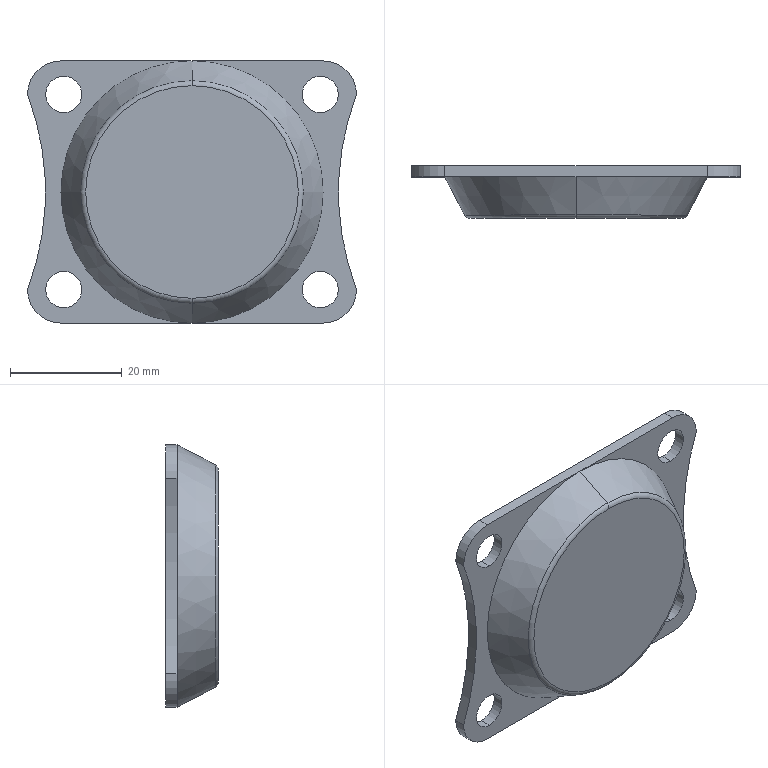Part | STEP file | CLGJ50_Rswivel | 1 solid | 27 faces | box 59 x 9.375 x 47 mm | volume 14515 mm3 | cylinder 16 | plane 7 | torus 2 | cone 2 | commonest cylinder face diameters 6.5 x8 12 x4 39.333 x2 98.33 x2
STEP:
#1=CARTESIAN_POINT('',(0.,-9.375,19.059));
#2=VERTEX_POINT('',#1);
#3=CARTESIAN_POINT('',(0.,-9.375,-19.059));
#4=VERTEX_POINT('',#3);
#5=CARTESIAN_POINT('',(0.,-9.375,0.));
#6=DIRECTION('',(0.,1.,0.));
#7=DIRECTION('',(0.,0.,1.));
#8=AXIS2_PLACEMENT_3D('',#5,#6,#7);
#9=CIRCLE('',#8,19.059);
#10=EDGE_CURVE('',#2,#4,#9,.T.);
#11=ORIENTED_EDGE('',*,*,#10,.T.);
#12=CARTESIAN_POINT('',(0.,-8.836,-19.947));
#13=VERTEX_POINT('',#12);
#14=CARTESIAN_POINT('',(0.,-8.375,-19.059));
#15=DIRECTION('',(1.,0.,0.));
#16=DIRECTION('',(0.,0.,-1.));
#17=AXIS2_PLACEMENT_3D('',#14,#15,#16);
#18=CIRCLE('',#17,1.);
#19=EDGE_CURVE('',#4,#13,#18,.T.);
#20=ORIENTED_EDGE('',*,*,#19,.T.);
#21=CARTESIAN_POINT('',(0.,-8.836,19.947));
#22=VERTEX_POINT('',#21);
#23=CARTESIAN_POINT('',(0.,-8.836,0.));
#24=DIRECTION('',(0.,1.,0.));
#25=DIRECTION('',(0.,0.,1.));
#26=AXIS2_PLACEMENT_3D('',#23,#24,#25);
#27=CIRCLE('',#26,19.947);
#28=EDGE_CURVE('',#22,#13,#27,.T.);
#29=ORIENTED_EDGE('',*,*,#28,.F.);
#30=CARTESIAN_POINT('',(0.,-8.375,19.059));
#31=DIRECTION('',(-1.,0.,0.));
#32=DIRECTION('',(0.,0.,1.));
#33=AXIS2_PLACEMENT_3D('',#30,#31,#32);
#34=CIRCLE('',#33,1.);
#35=EDGE_CURVE('',#2,#22,#34,.T.);
#36=ORIENTED_EDGE('',*,*,#35,.F.);
#37=EDGE_LOOP('',(#11,#20,#29,#36));
#38=FACE_OUTER_BOUND('',#37,.T.);
#39=CARTESIAN_POINT('',(0.,-8.375,0.));
#40=DIRECTION('',(0.,1.,0.));
#41=DIRECTION('',(0.,0.,1.));
#42=AXIS2_PLACEMENT_3D('',#39,#40,#41);
#43=TOROIDAL_SURFACE('',#42,19.059,1.);
#44=ADVANCED_FACE('',(#38),#43,.T.);
#45=ORIENTED_EDGE('',*,*,#28,.T.);
#46=CARTESIAN_POINT('',(0.,-2.,-23.5));
#47=VERTEX_POINT('',#46);
#48=CARTESIAN_POINT('',(0.,-8.836,-19.947));
#49=DIRECTION('',(0.,0.8873,-0.4612));
#50=VECTOR('',#49,1000.);
#51=LINE('',#48,#50);
#52=EDGE_CURVE('',#13,#47,#51,.T.);
#53=ORIENTED_EDGE('',*,*,#52,.T.);
#54=CARTESIAN_POINT('',(0.,-2.,23.5));
#55=VERTEX_POINT('',#54);
#56=CARTESIAN_POINT('',(0.,-2.,0.));
#57=DIRECTION('',(0.,1.,0.));
#58=DIRECTION('',(0.,0.,1.));
#59=AXIS2_PLACEMENT_3D('',#56,#57,#58);
#60=CIRCLE('',#59,23.5);
#61=EDGE_CURVE('',#55,#47,#60,.T.);
#62=ORIENTED_EDGE('',*,*,#61,.F.);
#63=CARTESIAN_POINT('',(0.,-8.836,19.947));
#64=DIRECTION('',(0.,0.8873,0.4612));
#65=VECTOR('',#64,1000.);
#66=LINE('',#63,#65);
#67=EDGE_CURVE('',#22,#55,#66,.T.);
#68=ORIENTED_EDGE('',*,*,#67,.F.);
#69=EDGE_LOOP('',(#45,#53,#62,#68));
#70=FACE_OUTER_BOUND('',#69,.T.);
#71=CARTESIAN_POINT('',(0.,-8.836,0.));
#72=DIRECTION('',(0.,1.,0.));
#73=DIRECTION('',(0.,0.,1.));
#74=AXIS2_PLACEMENT_3D('',#71,#72,#73);
#75=CONICAL_SURFACE('',#74,19.947,0.4793);
#76=ADVANCED_FACE('',(#70),#75,.T.);
#77=CARTESIAN_POINT('',(0.,-1.,-19.667));
#78=VERTEX_POINT('',#77);
#79=CARTESIAN_POINT('',(0.,-1.,19.667));
#80=VERTEX_POINT('',#79);
#81=CARTESIAN_POINT('',(0.,-1.,0.));
#82=DIRECTION('',(0.,1.,0.));
#83=DIRECTION('',(0.,0.,1.));
#84=AXIS2_PLACEMENT_3D('',#81,#82,#83);
#85=CIRCLE('',#84,19.667);
#86=EDGE_CURVE('',#78,#80,#85,.T.);
#87=ORIENTED_EDGE('',*,*,#86,.F.);
#88=CARTESIAN_POINT('',(0.,0.,-19.667));
#89=VERTEX_POINT('',#88);
#90=CARTESIAN_POINT('',(0.,-1.,-19.667));
#91=DIRECTION('',(0.,1.,0.));
#92=VECTOR('',#91,1000.);
#93=LINE('',#90,#92);
#94=EDGE_CURVE('',#78,#89,#93,.T.);
#95=ORIENTED_EDGE('',*,*,#94,.T.);
#96=CARTESIAN_POINT('',(0.,0.,19.667));
#97=VERTEX_POINT('',#96);
#98=CARTESIAN_POINT('',(0.,0.,0.));
#99=DIRECTION('',(0.,1.,0.));
#100=DIRECTION('',(0.,0.,1.));
#101=AXIS2_PLACEMENT_3D('',#98,#99,#100);
#102=CIRCLE('',#101,19.667);
#103=EDGE_CURVE('',#89,#97,#102,.T.);
#104=ORIENTED_EDGE('',*,*,#103,.T.);
#105=CARTESIAN_POINT('',(0.,-1.,19.667));
#106=DIRECTION('',(0.,1.,0.));
#107=VECTOR('',#106,1000.);
#108=LINE('',#105,#107);
#109=EDGE_CURVE('',#80,#97,#108,.T.);
#110=ORIENTED_EDGE('',*,*,#109,.F.);
#111=EDGE_LOOP('',(#87,#95,#104,#110));
#112=FACE_OUTER_BOUND('',#111,.T.);
#113=CARTESIAN_POINT('',(0.,-1.,0.));
#114=DIRECTION('',(0.,1.,0.));
#115=DIRECTION('',(0.,0.,1.));
#116=AXIS2_PLACEMENT_3D('',#113,#114,#115);
#117=CYLINDRICAL_SURFACE('',#116,19.667);
#118=ADVANCED_FACE('',(#112),#117,.F.);
#119=CARTESIAN_POINT('',(-23.,-2.,-20.75));
#120=VERTEX_POINT('',#119);
#121=CARTESIAN_POINT('',(-23.,-2.,-14.25));
#122=VERTEX_POINT('',#121);
#123=CARTESIAN_POINT('',(-23.,-2.,-17.5));
#124=DIRECTION('',(0.,1.,0.));
#125=DIRECTION('',(0.,0.,1.));
#126=AXIS2_PLACEMENT_3D('',#123,#124,#125);
#127=CIRCLE('',#126,3.25);
#128=EDGE_CURVE('',#120,#122,#127,.T.);
#129=ORIENTED_EDGE('',*,*,#128,.F.);
#130=CARTESIAN_POINT('',(-23.,0.,-20.75));
#131=VERTEX_POINT('',#130);
#132=CARTESIAN_POINT('',(-23.,-2.,-20.75));
#133=DIRECTION('',(0.,1.,0.));
#134=VECTOR('',#133,1000.);
#135=LINE('',#132,#134);
#136=EDGE_CURVE('',#120,#131,#135,.T.);
#137=ORIENTED_EDGE('',*,*,#136,.T.);
#138=CARTESIAN_POINT('',(-23.,0.,-14.25));
#139=VERTEX_POINT('',#138);
#140=CARTESIAN_POINT('',(-23.,0.,-17.5));
#141=DIRECTION('',(0.,1.,0.));
#142=DIRECTION('',(0.,0.,1.));
#143=AXIS2_PLACEMENT_3D('',#140,#141,#142);
#144=CIRCLE('',#143,3.25);
#145=EDGE_CURVE('',#131,#139,#144,.T.);
#146=ORIENTED_EDGE('',*,*,#145,.T.);
#147=CARTESIAN_POINT('',(-23.,-2.,-14.25));
#148=DIRECTION('',(0.,1.,0.));
#149=VECTOR('',#148,1000.);
#150=LINE('',#147,#149);
#151=EDGE_CURVE('',#122,#139,#150,.T.);
#152=ORIENTED_EDGE('',*,*,#151,.F.);
#153=EDGE_LOOP('',(#129,#137,#146,#152));
#154=FACE_OUTER_BOUND('',#153,.T.);
#155=CARTESIAN_POINT('',(-23.,-2.,-17.5));
#156=DIRECTION('',(0.,1.,0.));
#157=DIRECTION('',(0.,0.,1.));
#158=AXIS2_PLACEMENT_3D('',#155,#156,#157);
#159=CYLINDRICAL_SURFACE('',#158,3.25);
#160=ADVANCED_FACE('',(#154),#159,.F.);
#161=CARTESIAN_POINT('',(-23.,-2.,14.25));
#162=VERTEX_POINT('',#161);
#163=CARTESIAN_POINT('',(-23.,-2.,20.75));
#164=VERTEX_POINT('',#163);
#165=CARTESIAN_POINT('',(-23.,-2.,17.5));
#166=DIRECTION('',(0.,1.,0.));
#167=DIRECTION('',(0.,0.,1.));
#168=AXIS2_PLACEMENT_3D('',#165,#166,#167);
#169=CIRCLE('',#168,3.25);
#170=EDGE_CURVE('',#162,#164,#169,.T.);
#171=ORIENTED_EDGE('',*,*,#170,.F.);
#172=CARTESIAN_POINT('',(-23.,0.,14.25));
#173=VERTEX_POINT('',#172);
#174=CARTESIAN_POINT('',(-23.,-2.,14.25));
#175=DIRECTION('',(0.,1.,0.));
#176=VECTOR('',#175,1000.);
#177=LINE('',#174,#176);
#178=EDGE_CURVE('',#162,#173,#177,.T.);
#179=ORIENTED_EDGE('',*,*,#178,.T.);
#180=CARTESIAN_POINT('',(-23.,0.,20.75));
#181=VERTEX_POINT('',#180);
#182=CARTESIAN_POINT('',(-23.,0.,17.5));
#183=DIRECTION('',(0.,1.,0.));
#184=DIRECTION('',(0.,0.,1.));
#185=AXIS2_PLACEMENT_3D('',#182,#183,#184);
#186=CIRCLE('',#185,3.25);
#187=EDGE_CURVE('',#173,#181,#186,.T.);
#188=ORIENTED_EDGE('',*,*,#187,.T.);
#189=CARTESIAN_POINT('',(-23.,-2.,20.75));
#190=DIRECTION('',(0.,1.,0.));
#191=VECTOR('',#190,1000.);
#192=LINE('',#189,#191);
#193=EDGE_CURVE('',#164,#181,#192,.T.);
#194=ORIENTED_EDGE('',*,*,#193,.F.);
#195=EDGE_LOOP('',(#171,#179,#188,#194));
#196=FACE_OUTER_BOUND('',#195,.T.);
#197=CARTESIAN_POINT('',(-23.,-2.,17.5));
#198=DIRECTION('',(0.,1.,0.));
#199=DIRECTION('',(0.,0.,1.));
#200=AXIS2_PLACEMENT_3D('',#197,#198,#199);
#201=CYLINDRICAL_SURFACE('',#200,3.25);
#202=ADVANCED_FACE('',(#196),#201,.F.);
#203=CARTESIAN_POINT('',(23.,-2.,-20.75));
#204=VERTEX_POINT('',#203);
#205=CARTESIAN_POINT('',(23.,-2.,-14.25));
#206=VERTEX_POINT('',#205);
#207=CARTESIAN_POINT('',(23.,-2.,-17.5));
#208=DIRECTION('',(0.,1.,0.));
#209=DIRECTION('',(0.,0.,1.));
#210=AXIS2_PLACEMENT_3D('',#207,#208,#209);
#211=CIRCLE('',#210,3.25);
#212=EDGE_CURVE('',#204,#206,#211,.T.);
#213=ORIENTED_EDGE('',*,*,#212,.F.);
#214=CARTESIAN_POINT('',(23.,0.,-20.75));
#215=VERTEX_POINT('',#214);
#216=CARTESIAN_POINT('',(23.,-2.,-20.75));
#217=DIRECTION('',(0.,1.,0.));
#218=VECTOR('',#217,1000.);
#219=LINE('',#216,#218);
#220=EDGE_CURVE('',#204,#215,#219,.T.);
#221=ORIENTED_EDGE('',*,*,#220,.T.);
#222=CARTESIAN_POINT('',(23.,0.,-14.25));
#223=VERTEX_POINT('',#222);
#224=CARTESIAN_POINT('',(23.,0.,-17.5));
#225=DIRECTION('',(0.,1.,0.));
#226=DIRECTION('',(0.,0.,1.));
#227=AXIS2_PLACEMENT_3D('',#224,#225,#226);
#228=CIRCLE('',#227,3.25);
#229=EDGE_CURVE('',#215,#223,#228,.T.);
#230=ORIENTED_EDGE('',*,*,#229,.T.);
#231=CARTESIAN_POINT('',(23.,-2.,-14.25));
#232=DIRECTION('',(0.,1.,0.));
#233=VECTOR('',#232,1000.);
#234=LINE('',#231,#233);
#235=EDGE_CURVE('',#206,#223,#234,.T.);
#236=ORIENTED_EDGE('',*,*,#235,.F.);
#237=EDGE_LOOP('',(#213,#221,#230,#236));
#238=FACE_OUTER_BOUND('',#237,.T.);
#239=CARTESIAN_POINT('',(23.,-2.,-17.5));
#240=DIRECTION('',(0.,1.,0.));
#241=DIRECTION('',(0.,0.,1.));
#242=AXIS2_PLACEMENT_3D('',#239,#240,#241);
#243=CYLINDRICAL_SURFACE('',#242,3.25);
#244=ADVANCED_FACE('',(#238),#243,.F.);
#245=CARTESIAN_POINT('',(23.,-2.,14.25));
#246=VERTEX_POINT('',#245);
#247=CARTESIAN_POINT('',(23.,-2.,20.75));
#248=VERTEX_POINT('',#247);
#249=CARTESIAN_POINT('',(23.,-2.,17.5));
#250=DIRECTION('',(0.,1.,0.));
#251=DIRECTION('',(0.,0.,1.));
#252=AXIS2_PLACEMENT_3D('',#249,#250,#251);
#253=CIRCLE('',#252,3.25);
#254=EDGE_CURVE('',#246,#248,#253,.T.);
#255=ORIENTED_EDGE('',*,*,#254,.F.);
#256=CARTESIAN_POINT('',(23.,0.,14.25));
#257=VERTEX_POINT('',#256);
#258=CARTESIAN_POINT('',(23.,-2.,14.25));
#259=DIRECTION('',(0.,1.,0.));
#260=VECTOR('',#259,1000.);
#261=LINE('',#258,#260);
#262=EDGE_CURVE('',#246,#257,#261,.T.);
#263=ORIENTED_EDGE('',*,*,#262,.T.);
#264=CARTESIAN_POINT('',(23.,0.,20.75));
#265=VERTEX_POINT('',#264);
#266=CARTESIAN_POINT('',(23.,0.,17.5));
#267=DIRECTION('',(0.,1.,0.));
#268=DIRECTION('',(0.,0.,1.));
#269=AXIS2_PLACEMENT_3D('',#266,#267,#268);
#270=CIRCLE('',#269,3.25);
#271=EDGE_CURVE('',#257,#265,#270,.T.);
#272=ORIENTED_EDGE('',*,*,#271,.T.);
#273=CARTESIAN_POINT('',(23.,-2.,20.75));
#274=DIRECTION('',(0.,1.,0.));
#275=VECTOR('',#274,1000.);
#276=LINE('',#273,#275);
#277=EDGE_CURVE('',#248,#265,#276,.T.);
#278=ORIENTED_EDGE('',*,*,#277,.F.);
#279=EDGE_LOOP('',(#255,#263,#272,#278));
#280=FACE_OUTER_BOUND('',#279,.T.);
#281=CARTESIAN_POINT('',(23.,-2.,17.5));
#282=DIRECTION('',(0.,1.,0.));
#283=DIRECTION('',(0.,0.,1.));
#284=AXIS2_PLACEMENT_3D('',#281,#282,#283);
#285=CYLINDRICAL_SURFACE('',#284,3.25);
#286=ADVANCED_FACE('',(#280),#285,.F.);
#287=CARTESIAN_POINT('',(23.,-2.,17.5));
#288=DIRECTION('',(0.,1.,0.));
#289=DIRECTION('',(0.,0.,1.));
#290=AXIS2_PLACEMENT_3D('',#287,#288,#289);
#291=CIRCLE('',#290,3.25);
#292=EDGE_CURVE('',#248,#246,#291,.T.);
#293=ORIENTED_EDGE('',*,*,#292,.T.);
#294=ORIENTED_EDGE('',*,*,#254,.T.);
#295=EDGE_LOOP('',(#293,#294));
#296=FACE_BOUND('',#295,.T.);
#297=CARTESIAN_POINT('',(23.,-2.,-17.5));
#298=DIRECTION('',(0.,1.,0.));
#299=DIRECTION('',(0.,0.,1.));
#300=AXIS2_PLACEMENT_3D('',#297,#298,#299);
#301=CIRCLE('',#300,3.25);
#302=EDGE_CURVE('',#206,#204,#301,.T.);
#303=ORIENTED_EDGE('',*,*,#302,.T.);
#304=ORIENTED_EDGE('',*,*,#212,.T.);
#305=EDGE_LOOP('',(#303,#304));
#306=FACE_BOUND('',#305,.T.);
#307=CARTESIAN_POINT('',(23.5,-2.,23.5));
#308=VERTEX_POINT('',#307);
#309=CARTESIAN_POINT('',(-23.5,-2.,23.5));
#310=DIRECTION('',(1.,0.,0.));
#311=VECTOR('',#310,1000.);
#312=LINE('',#309,#311);
#313=EDGE_CURVE('',#55,#308,#312,.T.);
#314=ORIENTED_EDGE('',*,*,#313,.F.);
#315=ORIENTED_EDGE('',*,*,#61,.T.);
#316=CARTESIAN_POINT('',(23.5,-2.,-23.5));
#317=VERTEX_POINT('',#316);
#318=CARTESIAN_POINT('',(23.5,-2.,-23.5));
#319=DIRECTION('',(-1.,0.,0.));
#320=VECTOR('',#319,1000.);
#321=LINE('',#318,#320);
#322=EDGE_CURVE('',#317,#47,#321,.T.);
#323=ORIENTED_EDGE('',*,*,#322,.F.);
#324=CARTESIAN_POINT('',(29.5,-2.,-17.5));
#325=VERTEX_POINT('',#324);
#326=CARTESIAN_POINT('',(23.5,-2.,-17.5));
#327=DIRECTION('',(0.,1.,0.));
#328=DIRECTION('',(0.,0.,1.));
#329=AXIS2_PLACEMENT_3D('',#326,#327,#328);
#330=CIRCLE('',#329,6.);
#331=EDGE_CURVE('',#325,#317,#330,.T.);
#332=ORIENTED_EDGE('',*,*,#331,.F.);
#333=CARTESIAN_POINT('',(29.5,-2.,17.5));
#334=VERTEX_POINT('',#333);
#335=CARTESIAN_POINT('',(75.445,-2.,0.));
#336=DIRECTION('',(0.,-1.,0.));
#337=DIRECTION('',(0.,0.,-1.));
#338=AXIS2_PLACEMENT_3D('',#335,#336,#337);
#339=CIRCLE('',#338,49.165);
#340=EDGE_CURVE('',#334,#325,#339,.T.);
#341=ORIENTED_EDGE('',*,*,#340,.F.);
#342=CARTESIAN_POINT('',(23.5,-2.,17.5));
#343=DIRECTION('',(0.,1.,0.));
#344=DIRECTION('',(0.,0.,1.));
#345=AXIS2_PLACEMENT_3D('',#342,#343,#344);
#346=CIRCLE('',#345,6.);
#347=EDGE_CURVE('',#308,#334,#346,.T.);
#348=ORIENTED_EDGE('',*,*,#347,.F.);
#349=EDGE_LOOP('',(#314,#315,#323,#332,#341,#348));
#350=FACE_OUTER_BOUND('',#349,.T.);
#351=CARTESIAN_POINT('',(-23.5,-2.,-17.5));
#352=DIRECTION('',(0.,1.,0.));
#353=DIRECTION('',(0.,0.,1.));
#354=AXIS2_PLACEMENT_3D('',#351,#352,#353);
#355=PLANE('',#354);
#356=ADVANCED_FACE('',(#296,#306,#350),#355,.F.);
#357=CARTESIAN_POINT('',(-23.5,0.,-23.5));
#358=VERTEX_POINT('',#357);
#359=CARTESIAN_POINT('',(-29.5,0.,-17.5));
#360=VERTEX_POINT('',#359);
#361=CARTESIAN_POINT('',(-23.5,0.,-17.5));
#362=DIRECTION('',(0.,1.,0.));
#363=DIRECTION('',(0.,0.,1.));
#364=AXIS2_PLACEMENT_3D('',#361,#362,#363);
#365=CIRCLE('',#364,6.);
#366=EDGE_CURVE('',#358,#360,#365,.T.);
#367=ORIENTED_EDGE('',*,*,#366,.F.);
#368=CARTESIAN_POINT('',(-23.5,-2.,-23.5));
#369=VERTEX_POINT('',#368);
#370=CARTESIAN_POINT('',(-23.5,-2.,-23.5));
#371=DIRECTION('',(0.,1.,0.));
#372=VECTOR('',#371,1000.);
#373=LINE('',#370,#372);
#374=EDGE_CURVE('',#369,#358,#373,.T.);
#375=ORIENTED_EDGE('',*,*,#374,.F.);
#376=CARTESIAN_POINT('',(-29.5,-2.,-17.5));
#377=VERTEX_POINT('',#376);
#378=CARTESIAN_POINT('',(-23.5,-2.,-17.5));
#379=DIRECTION('',(0.,1.,0.));
#380=DIRECTION('',(0.,0.,1.));
#381=AXIS2_PLACEMENT_3D('',#378,#379,#380);
#382=CIRCLE('',#381,6.);
#383=EDGE_CURVE('',#369,#377,#382,.T.);
#384=ORIENTED_EDGE('',*,*,#383,.T.);
#385=CARTESIAN_POINT('',(-29.5,-2.,-17.5));
#386=DIRECTION('',(0.,1.,0.));
#387=VECTOR('',#386,1000.);
#388=LINE('',#385,#387);
#389=EDGE_CURVE('',#377,#360,#388,.T.);
#390=ORIENTED_EDGE('',*,*,#389,.T.);
#391=EDGE_LOOP('',(#367,#375,#384,#390));
#392=FACE_OUTER_BOUND('',#391,.T.);
#393=CARTESIAN_POINT('',(-23.5,-2.,-17.5));
#394=DIRECTION('',(0.,1.,0.));
#395=DIRECTION('',(0.,0.,1.));
#396=AXIS2_PLACEMENT_3D('',#393,#394,#395);
#397=CYLINDRICAL_SURFACE('',#396,6.);
#398=ADVANCED_FACE('',(#392),#397,.T.);
#399=CARTESIAN_POINT('',(23.5,0.,-23.5));
#400=VERTEX_POINT('',#399);
#401=CARTESIAN_POINT('',(23.5,0.,-23.5));
#402=DIRECTION('',(-1.,0.,0.));
#403=VECTOR('',#402,1000.);
#404=LINE('',#401,#403);
#405=EDGE_CURVE('',#400,#358,#404,.T.);
#406=ORIENTED_EDGE('',*,*,#405,.F.);
#407=CARTESIAN_POINT('',(23.5,-2.,-23.5));
#408=DIRECTION('',(0.,1.,0.));
#409=VECTOR('',#408,1000.);
#410=LINE('',#407,#409);
#411=EDGE_CURVE('',#317,#400,#410,.T.);
#412=ORIENTED_EDGE('',*,*,#411,.F.);
#413=ORIENTED_EDGE('',*,*,#322,.T.);
#414=CARTESIAN_POINT('',(23.5,-2.,-23.5));
#415=DIRECTION('',(-1.,0.,0.));
#416=VECTOR('',#415,1000.);
#417=LINE('',#414,#416);
#418=EDGE_CURVE('',#47,#369,#417,.T.);
#419=ORIENTED_EDGE('',*,*,#418,.T.);
#420=ORIENTED_EDGE('',*,*,#374,.T.);
#421=EDGE_LOOP('',(#406,#412,#413,#419,#420));
#422=FACE_OUTER_BOUND('',#421,.T.);
#423=CARTESIAN_POINT('',(23.5,-2.,-23.5));
#424=DIRECTION('',(0.,0.,-1.));
#425=DIRECTION('',(-1.,0.,0.));
#426=AXIS2_PLACEMENT_3D('',#423,#424,#425);
#427=PLANE('',#426);
#428=ADVANCED_FACE('',(#422),#427,.T.);
#429=CARTESIAN_POINT('',(29.5,0.,-17.5));
#430=VERTEX_POINT('',#429);
#431=CARTESIAN_POINT('',(23.5,0.,-17.5));
#432=DIRECTION('',(0.,1.,0.));
#433=DIRECTION('',(0.,0.,1.));
#434=AXIS2_PLACEMENT_3D('',#431,#432,#433);
#435=CIRCLE('',#434,6.);
#436=EDGE_CURVE('',#430,#400,#435,.T.);
#437=ORIENTED_EDGE('',*,*,#436,.F.);
#438=CARTESIAN_POINT('',(29.5,-2.,-17.5));
#439=DIRECTION('',(0.,1.,0.));
#440=VECTOR('',#439,1000.);
#441=LINE('',#438,#440);
#442=EDGE_CURVE('',#325,#430,#441,.T.);
#443=ORIENTED_EDGE('',*,*,#442,.F.);
#444=ORIENTED_EDGE('',*,*,#331,.T.);
#445=ORIENTED_EDGE('',*,*,#411,.T.);
#446=EDGE_LOOP('',(#437,#443,#444,#445));
#447=FACE_OUTER_BOUND('',#446,.T.);
#448=CARTESIAN_POINT('',(23.5,-2.,-17.5));
#449=DIRECTION('',(0.,1.,0.));
#450=DIRECTION('',(0.,0.,1.));
#451=AXIS2_PLACEMENT_3D('',#448,#449,#450);
#452=CYLINDRICAL_SURFACE('',#451,6.);
#453=ADVANCED_FACE('',(#447),#452,.T.);
#454=CARTESIAN_POINT('',(29.5,0.,17.5));
#455=VERTEX_POINT('',#454);
#456=CARTESIAN_POINT('',(75.445,0.,0.));
#457=DIRECTION('',(0.,-1.,0.));
#458=DIRECTION('',(0.,0.,-1.));
#459=AXIS2_PLACEMENT_3D('',#456,#457,#458);
#460=CIRCLE('',#459,49.165);
#461=EDGE_CURVE('',#455,#430,#460,.T.);
#462=ORIENTED_EDGE('',*,*,#461,.F.);
#463=CARTESIAN_POINT('',(29.5,-2.,17.5));
#464=DIRECTION('',(0.,1.,0.));
#465=VECTOR('',#464,1000.);
#466=LINE('',#463,#465);
#467=EDGE_CURVE('',#334,#455,#466,.T.);
#468=ORIENTED_EDGE('',*,*,#467,.F.);
#469=ORIENTED_EDGE('',*,*,#340,.T.);
#470=ORIENTED_EDGE('',*,*,#442,.T.);
#471=EDGE_LOOP('',(#462,#468,#469,#470));
#472=FACE_OUTER_BOUND('',#471,.T.);
#473=CARTESIAN_POINT('',(75.445,-2.,0.));
#474=DIRECTION('',(0.,1.,0.));
#475=DIRECTION('',(0.,0.,1.));
#476=AXIS2_PLACEMENT_3D('',#473,#474,#475);
#477=CYLINDRICAL_SURFACE('',#476,49.165);
#478=ADVANCED_FACE('',(#472),#477,.F.);
#479=CARTESIAN_POINT('',(23.5,0.,23.5));
#480=VERTEX_POINT('',#479);
#481=CARTESIAN_POINT('',(23.5,0.,17.5));
#482=DIRECTION('',(0.,1.,0.));
#483=DIRECTION('',(0.,0.,1.));
#484=AXIS2_PLACEMENT_3D('',#481,#482,#483);
#485=CIRCLE('',#484,6.);
#486=EDGE_CURVE('',#480,#455,#485,.T.);
#487=ORIENTED_EDGE('',*,*,#486,.F.);
#488=CARTESIAN_POINT('',(23.5,-2.,23.5));
#489=DIRECTION('',(0.,1.,0.));
#490=VECTOR('',#489,1000.);
#491=LINE('',#488,#490);
#492=EDGE_CURVE('',#308,#480,#491,.T.);
#493=ORIENTED_EDGE('',*,*,#492,.F.);
#494=ORIENTED_EDGE('',*,*,#347,.T.);
#495=ORIENTED_EDGE('',*,*,#467,.T.);
#496=EDGE_LOOP('',(#487,#493,#494,#495));
#497=FACE_OUTER_BOUND('',#496,.T.);
#498=CARTESIAN_POINT('',(23.5,-2.,17.5));
#499=DIRECTION('',(0.,1.,0.));
#500=DIRECTION('',(0.,0.,1.));
#501=AXIS2_PLACEMENT_3D('',#498,#499,#500);
#502=CYLINDRICAL_SURFACE('',#501,6.);
#503=ADVANCED_FACE('',(#497),#502,.T.);
#504=CARTESIAN_POINT('',(-23.5,0.,23.5));
#505=VERTEX_POINT('',#504);
#506=CARTESIAN_POINT('',(-23.5,0.,23.5));
#507=DIRECTION('',(1.,0.,0.));
#508=VECTOR('',#507,1000.);
#509=LINE('',#506,#508);
#510=EDGE_CURVE('',#505,#480,#509,.T.);
#511=ORIENTED_EDGE('',*,*,#510,.F.);
#512=CARTESIAN_POINT('',(-23.5,-2.,23.5));
#513=VERTEX_POINT('',#512);
#514=CARTESIAN_POINT('',(-23.5,-2.,23.5));
#515=DIRECTION('',(0.,1.,0.));
#516=VECTOR('',#515,1000.);
#517=LINE('',#514,#516);
#518=EDGE_CURVE('',#513,#505,#517,.T.);
#519=ORIENTED_EDGE('',*,*,#518,.F.);
#520=CARTESIAN_POINT('',(-23.5,-2.,23.5));
#521=DIRECTION('',(1.,0.,0.));
#522=VECTOR('',#521,1000.);
#523=LINE('',#520,#522);
#524=EDGE_CURVE('',#513,#55,#523,.T.);
#525=ORIENTED_EDGE('',*,*,#524,.T.);
#526=ORIENTED_EDGE('',*,*,#313,.T.);
#527=ORIENTED_EDGE('',*,*,#492,.T.);
#528=EDGE_LOOP('',(#511,#519,#525,#526,#527));
#529=FACE_OUTER_BOUND('',#528,.T.);
#530=CARTESIAN_POINT('',(-23.5,-2.,23.5));
#531=DIRECTION('',(0.,0.,1.));
#532=DIRECTION('',(1.,0.,0.));
#533=AXIS2_PLACEMENT_3D('',#530,#531,#532);
#534=PLANE('',#533);
#535=ADVANCED_FACE('',(#529),#534,.T.);
#536=CARTESIAN_POINT('',(-29.5,0.,17.5));
#537=VERTEX_POINT('',#536);
#538=CARTESIAN_POINT('',(-23.5,0.,17.5));
#539=DIRECTION('',(0.,1.,0.));
#540=DIRECTION('',(0.,0.,1.));
#541=AXIS2_PLACEMENT_3D('',#538,#539,#540);
#542=CIRCLE('',#541,6.);
#543=EDGE_CURVE('',#537,#505,#542,.T.);
#544=ORIENTED_EDGE('',*,*,#543,.F.);
#545=CARTESIAN_POINT('',(-29.5,-2.,17.5));
#546=VERTEX_POINT('',#545);
#547=CARTESIAN_POINT('',(-29.5,-2.,17.5));
#548=DIRECTION('',(0.,1.,0.));
#549=VECTOR('',#548,1000.);
#550=LINE('',#547,#549);
#551=EDGE_CURVE('',#546,#537,#550,.T.);
#552=ORIENTED_EDGE('',*,*,#551,.F.);
#553=CARTESIAN_POINT('',(-23.5,-2.,17.5));
#554=DIRECTION('',(0.,1.,0.));
#555=DIRECTION('',(0.,0.,1.));
#556=AXIS2_PLACEMENT_3D('',#553,#554,#555);
#557=CIRCLE('',#556,6.);
#558=EDGE_CURVE('',#546,#513,#557,.T.);
#559=ORIENTED_EDGE('',*,*,#558,.T.);
#560=ORIENTED_EDGE('',*,*,#518,.T.);
#561=EDGE_LOOP('',(#544,#552,#559,#560));
#562=FACE_OUTER_BOUND('',#561,.T.);
#563=CARTESIAN_POINT('',(-23.5,-2.,17.5));
#564=DIRECTION('',(0.,1.,0.));
#565=DIRECTION('',(0.,0.,1.));
#566=AXIS2_PLACEMENT_3D('',#563,#564,#565);
#567=CYLINDRICAL_SURFACE('',#566,6.);
#568=ADVANCED_FACE('',(#562),#567,.T.);
#569=CARTESIAN_POINT('',(-75.445,0.,0.));
#570=DIRECTION('',(0.,-1.,0.));
#571=DIRECTION('',(0.,0.,-1.));
#572=AXIS2_PLACEMENT_3D('',#569,#570,#571);
#573=CIRCLE('',#572,49.165);
#574=EDGE_CURVE('',#360,#537,#573,.T.);
#575=ORIENTED_EDGE('',*,*,#574,.F.);
#576=ORIENTED_EDGE('',*,*,#389,.F.);
#577=CARTESIAN_POINT('',(-75.445,-2.,0.));
#578=DIRECTION('',(0.,-1.,0.));
#579=DIRECTION('',(0.,0.,-1.));
#580=AXIS2_PLACEMENT_3D('',#577,#578,#579);
#581=CIRCLE('',#580,49.165);
#582=EDGE_CURVE('',#377,#546,#581,.T.);
#583=ORIENTED_EDGE('',*,*,#582,.T.);
#584=ORIENTED_EDGE('',*,*,#551,.T.);
#585=EDGE_LOOP('',(#575,#576,#583,#584));
#586=FACE_OUTER_BOUND('',#585,.T.);
#587=CARTESIAN_POINT('',(-75.445,-2.,0.));
#588=DIRECTION('',(0.,1.,0.));
#589=DIRECTION('',(0.,0.,1.));
#590=AXIS2_PLACEMENT_3D('',#587,#588,#589);
#591=CYLINDRICAL_SURFACE('',#590,49.165);
#592=ADVANCED_FACE('',(#586),#591,.F.);
#593=CARTESIAN_POINT('',(-23.,-2.,-17.5));
#594=DIRECTION('',(0.,1.,0.));
#595=DIRECTION('',(0.,0.,1.));
#596=AXIS2_PLACEMENT_3D('',#593,#594,#595);
#597=CIRCLE('',#596,3.25);
#598=EDGE_CURVE('',#122,#120,#597,.T.);
#599=ORIENTED_EDGE('',*,*,#598,.T.);
#600=ORIENTED_EDGE('',*,*,#128,.T.);
#601=EDGE_LOOP('',(#599,#600));
#602=FACE_BOUND('',#601,.T.);
#603=CARTESIAN_POINT('',(-23.,-2.,17.5));
#604=DIRECTION('',(0.,1.,0.));
#605=DIRECTION('',(0.,0.,1.));
#606=AXIS2_PLACEMENT_3D('',#603,#604,#605);
#607=CIRCLE('',#606,3.25);
#608=EDGE_CURVE('',#164,#162,#607,.T.);
#609=ORIENTED_EDGE('',*,*,#608,.T.);
#610=ORIENTED_EDGE('',*,*,#170,.T.);
#611=EDGE_LOOP('',(#609,#610));
#612=FACE_BOUND('',#611,.T.);
#613=ORIENTED_EDGE('',*,*,#418,.F.);
#614=CARTESIAN_POINT('',(0.,-2.,0.));
#615=DIRECTION('',(0.,1.,0.));
#616=DIRECTION('',(0.,0.,1.));
#617=AXIS2_PLACEMENT_3D('',#614,#615,#616);
#618=CIRCLE('',#617,23.5);
#619=EDGE_CURVE('',#47,#55,#618,.T.);
#620=ORIENTED_EDGE('',*,*,#619,.T.);
#621=ORIENTED_EDGE('',*,*,#524,.F.);
#622=ORIENTED_EDGE('',*,*,#558,.F.);
#623=ORIENTED_EDGE('',*,*,#582,.F.);
#624=ORIENTED_EDGE('',*,*,#383,.F.);
#625=EDGE_LOOP('',(#613,#620,#621,#622,#623,#624));
#626=FACE_OUTER_BOUND('',#625,.T.);
#627=CARTESIAN_POINT('',(-23.5,-2.,-17.5));
#628=DIRECTION('',(0.,1.,0.));
#629=DIRECTION('',(0.,0.,1.));
#630=AXIS2_PLACEMENT_3D('',#627,#628,#629);
#631=PLANE('',#630);
#632=ADVANCED_FACE('',(#602,#612,#626),#631,.F.);
#633=CARTESIAN_POINT('',(0.,0.,0.));
#634=DIRECTION('',(0.,1.,0.));
#635=DIRECTION('',(0.,0.,1.));
#636=AXIS2_PLACEMENT_3D('',#633,#634,#635);
#637=CIRCLE('',#636,19.667);
#638=EDGE_CURVE('',#97,#89,#637,.T.);
#639=ORIENTED_EDGE('',*,*,#638,.F.);
#640=ORIENTED_EDGE('',*,*,#103,.F.);
#641=EDGE_LOOP('',(#639,#640));
#642=FACE_BOUND('',#641,.T.);
#643=CARTESIAN_POINT('',(-23.,0.,-17.5));
#644=DIRECTION('',(0.,1.,0.));
#645=DIRECTION('',(0.,0.,1.));
#646=AXIS2_PLACEMENT_3D('',#643,#644,#645);
#647=CIRCLE('',#646,3.25);
#648=EDGE_CURVE('',#139,#131,#647,.T.);
#649=ORIENTED_EDGE('',*,*,#648,.F.);
#650=ORIENTED_EDGE('',*,*,#145,.F.);
#651=EDGE_LOOP('',(#649,#650));
#652=FACE_BOUND('',#651,.T.);
#653=CARTESIAN_POINT('',(-23.,0.,17.5));
#654=DIRECTION('',(0.,1.,0.));
#655=DIRECTION('',(0.,0.,1.));
#656=AXIS2_PLACEMENT_3D('',#653,#654,#655);
#657=CIRCLE('',#656,3.25);
#658=EDGE_CURVE('',#181,#173,#657,.T.);
#659=ORIENTED_EDGE('',*,*,#658,.F.);
#660=ORIENTED_EDGE('',*,*,#187,.F.);
#661=EDGE_LOOP('',(#659,#660));
#662=FACE_BOUND('',#661,.T.);
#663=CARTESIAN_POINT('',(23.,0.,-17.5));
#664=DIRECTION('',(0.,1.,0.));
#665=DIRECTION('',(0.,0.,1.));
#666=AXIS2_PLACEMENT_3D('',#663,#664,#665);
#667=CIRCLE('',#666,3.25);
#668=EDGE_CURVE('',#223,#215,#667,.T.);
#669=ORIENTED_EDGE('',*,*,#668,.F.);
#670=ORIENTED_EDGE('',*,*,#229,.F.);
#671=EDGE_LOOP('',(#669,#670));
#672=FACE_BOUND('',#671,.T.);
#673=CARTESIAN_POINT('',(23.,0.,17.5));
#674=DIRECTION('',(0.,1.,0.));
#675=DIRECTION('',(0.,0.,1.));
#676=AXIS2_PLACEMENT_3D('',#673,#674,#675);
#677=CIRCLE('',#676,3.25);
#678=EDGE_CURVE('',#265,#257,#677,.T.);
#679=ORIENTED_EDGE('',*,*,#678,.F.);
#680=ORIENTED_EDGE('',*,*,#271,.F.);
#681=EDGE_LOOP('',(#679,#680));
#682=FACE_BOUND('',#681,.T.);
#683=ORIENTED_EDGE('',*,*,#366,.T.);
#684=ORIENTED_EDGE('',*,*,#574,.T.);
#685=ORIENTED_EDGE('',*,*,#543,.T.);
#686=ORIENTED_EDGE('',*,*,#510,.T.);
#687=ORIENTED_EDGE('',*,*,#486,.T.);
#688=ORIENTED_EDGE('',*,*,#461,.T.);
#689=ORIENTED_EDGE('',*,*,#436,.T.);
#690=ORIENTED_EDGE('',*,*,#405,.T.);
#691=EDGE_LOOP('',(#683,#684,#685,#686,#687,#688,#689,#690));
#692=FACE_OUTER_BOUND('',#691,.T.);
#693=CARTESIAN_POINT('',(-23.5,0.,-17.5));
#694=DIRECTION('',(0.,1.,0.));
#695=DIRECTION('',(0.,0.,1.));
#696=AXIS2_PLACEMENT_3D('',#693,#694,#695);
#697=PLANE('',#696);
#698=ADVANCED_FACE('',(#642,#652,#662,#672,#682,#692),#697,.T.);
#699=ORIENTED_EDGE('',*,*,#262,.F.);
#700=ORIENTED_EDGE('',*,*,#292,.F.);
#701=ORIENTED_EDGE('',*,*,#277,.T.);
#702=ORIENTED_EDGE('',*,*,#678,.T.);
#703=EDGE_LOOP('',(#699,#700,#701,#702));
#704=FACE_OUTER_BOUND('',#703,.T.);
#705=CARTESIAN_POINT('',(23.,-2.,17.5));
#706=DIRECTION('',(0.,1.,0.));
#707=DIRECTION('',(0.,0.,1.));
#708=AXIS2_PLACEMENT_3D('',#705,#706,#707);
#709=CYLINDRICAL_SURFACE('',#708,3.25);
#710=ADVANCED_FACE('',(#704),#709,.F.);
#711=ORIENTED_EDGE('',*,*,#220,.F.);
#712=ORIENTED_EDGE('',*,*,#302,.F.);
#713=ORIENTED_EDGE('',*,*,#235,.T.);
#714=ORIENTED_EDGE('',*,*,#668,.T.);
#715=EDGE_LOOP('',(#711,#712,#713,#714));
#716=FACE_OUTER_BOUND('',#715,.T.);
#717=CARTESIAN_POINT('',(23.,-2.,-17.5));
#718=DIRECTION('',(0.,1.,0.));
#719=DIRECTION('',(0.,0.,1.));
#720=AXIS2_PLACEMENT_3D('',#717,#718,#719);
#721=CYLINDRICAL_SURFACE('',#720,3.25);
#722=ADVANCED_FACE('',(#716),#721,.F.);
#723=ORIENTED_EDGE('',*,*,#178,.F.);
#724=ORIENTED_EDGE('',*,*,#608,.F.);
#725=ORIENTED_EDGE('',*,*,#193,.T.);
#726=ORIENTED_EDGE('',*,*,#658,.T.);
#727=EDGE_LOOP('',(#723,#724,#725,#726));
#728=FACE_OUTER_BOUND('',#727,.T.);
#729=CARTESIAN_POINT('',(-23.,-2.,17.5));
#730=DIRECTION('',(0.,1.,0.));
#731=DIRECTION('',(0.,0.,1.));
#732=AXIS2_PLACEMENT_3D('',#729,#730,#731);
#733=CYLINDRICAL_SURFACE('',#732,3.25);
#734=ADVANCED_FACE('',(#728),#733,.F.);
#735=ORIENTED_EDGE('',*,*,#136,.F.);
#736=ORIENTED_EDGE('',*,*,#598,.F.);
#737=ORIENTED_EDGE('',*,*,#151,.T.);
#738=ORIENTED_EDGE('',*,*,#648,.T.);
#739=EDGE_LOOP('',(#735,#736,#737,#738));
#740=FACE_OUTER_BOUND('',#739,.T.);
#741=CARTESIAN_POINT('',(-23.,-2.,-17.5));
#742=DIRECTION('',(0.,1.,0.));
#743=DIRECTION('',(0.,0.,1.));
#744=AXIS2_PLACEMENT_3D('',#741,#742,#743);
#745=CYLINDRICAL_SURFACE('',#744,3.25);
#746=ADVANCED_FACE('',(#740),#745,.F.);
#747=ORIENTED_EDGE('',*,*,#94,.F.);
#748=CARTESIAN_POINT('',(0.,-1.,0.));
#749=DIRECTION('',(0.,1.,0.));
#750=DIRECTION('',(0.,0.,1.));
#751=AXIS2_PLACEMENT_3D('',#748,#749,#750);
#752=CIRCLE('',#751,19.667);
#753=EDGE_CURVE('',#80,#78,#752,.T.);
#754=ORIENTED_EDGE('',*,*,#753,.F.);
#755=ORIENTED_EDGE('',*,*,#109,.T.);
#756=ORIENTED_EDGE('',*,*,#638,.T.);
#757=EDGE_LOOP('',(#747,#754,#755,#756));
#758=FACE_OUTER_BOUND('',#757,.T.);
#759=CARTESIAN_POINT('',(0.,-1.,0.));
#760=DIRECTION('',(0.,1.,0.));
#761=DIRECTION('',(0.,0.,1.));
#762=AXIS2_PLACEMENT_3D('',#759,#760,#761);
#763=CYLINDRICAL_SURFACE('',#762,19.667);
#764=ADVANCED_FACE('',(#758),#763,.F.);
#765=ORIENTED_EDGE('',*,*,#753,.T.);
#766=ORIENTED_EDGE('',*,*,#86,.T.);
#767=EDGE_LOOP('',(#765,#766));
#768=FACE_OUTER_BOUND('',#767,.T.);
#769=CARTESIAN_POINT('',(0.,-1.,0.));
#770=DIRECTION('',(0.,1.,0.));
#771=DIRECTION('',(0.,0.,1.));
#772=AXIS2_PLACEMENT_3D('',#769,#770,#771);
#773=PLANE('',#772);
#774=ADVANCED_FACE('',(#768),#773,.T.);
#775=ORIENTED_EDGE('',*,*,#52,.F.);
#776=CARTESIAN_POINT('',(0.,-8.836,0.));
#777=DIRECTION('',(0.,1.,0.));
#778=DIRECTION('',(0.,0.,1.));
#779=AXIS2_PLACEMENT_3D('',#776,#777,#778);
#780=CIRCLE('',#779,19.947);
#781=EDGE_CURVE('',#13,#22,#780,.T.);
#782=ORIENTED_EDGE('',*,*,#781,.T.);
#783=ORIENTED_EDGE('',*,*,#67,.T.);
#784=ORIENTED_EDGE('',*,*,#619,.F.);
#785=EDGE_LOOP('',(#775,#782,#783,#784));
#786=FACE_OUTER_BOUND('',#785,.T.);
#787=CARTESIAN_POINT('',(0.,-8.836,0.));
#788=DIRECTION('',(0.,1.,0.));
#789=DIRECTION('',(0.,0.,1.));
#790=AXIS2_PLACEMENT_3D('',#787,#788,#789);
#791=CONICAL_SURFACE('',#790,19.947,0.4793);
#792=ADVANCED_FACE('',(#786),#791,.T.);
#793=ORIENTED_EDGE('',*,*,#19,.F.);
#794=CARTESIAN_POINT('',(0.,-9.375,0.));
#795=DIRECTION('',(0.,1.,0.));
#796=DIRECTION('',(0.,0.,1.));
#797=AXIS2_PLACEMENT_3D('',#794,#795,#796);
#798=CIRCLE('',#797,19.059);
#799=EDGE_CURVE('',#4,#2,#798,.T.);
#800=ORIENTED_EDGE('',*,*,#799,.T.);
#801=ORIENTED_EDGE('',*,*,#35,.T.);
#802=ORIENTED_EDGE('',*,*,#781,.F.);
#803=EDGE_LOOP('',(#793,#800,#801,#802));
#804=FACE_OUTER_BOUND('',#803,.T.);
#805=CARTESIAN_POINT('',(0.,-8.375,0.));
#806=DIRECTION('',(0.,1.,0.));
#807=DIRECTION('',(0.,0.,1.));
#808=AXIS2_PLACEMENT_3D('',#805,#806,#807);
#809=TOROIDAL_SURFACE('',#808,19.059,1.);
#810=ADVANCED_FACE('',(#804),#809,.T.);
#811=ORIENTED_EDGE('',*,*,#10,.F.);
#812=ORIENTED_EDGE('',*,*,#799,.F.);
#813=EDGE_LOOP('',(#811,#812));
#814=FACE_OUTER_BOUND('',#813,.T.);
#815=CARTESIAN_POINT('',(19.059,-9.375,0.));
#816=DIRECTION('',(0.,1.,0.));
#817=DIRECTION('',(0.,0.,1.));
#818=AXIS2_PLACEMENT_3D('',#815,#816,#817);
#819=PLANE('',#818);
#820=ADVANCED_FACE('',(#814),#819,.F.);
#821=CLOSED_SHELL('',(#44,#76,#118,#160,#202,#244,#286,#356,#398,#428,#453,#478,#503,#535,#568,#592,#632,#698,#710,#722,#734,#746,#764,#774,#792,#810,#820));
#822=MANIFOLD_SOLID_BREP('',#821);
#823=CARTESIAN_POINT('',(0.,0.,0.));
#824=DIRECTION('',(0.,0.,1.));
#825=DIRECTION('',(1.,0.,0.));
#826=AXIS2_PLACEMENT_3D('',#823,#824,#825);
#827=(LENGTH_UNIT()NAMED_UNIT(*)SI_UNIT(.MILLI.,.METRE.));
#828=UNCERTAINTY_MEASURE_WITH_UNIT(LENGTH_MEASURE(0.00001),#827,'','');
#829=(NAMED_UNIT(*)PLANE_ANGLE_UNIT()SI_UNIT($,.RADIAN.));
#830=(NAMED_UNIT(*)SI_UNIT($,.STERADIAN.)SOLID_ANGLE_UNIT());
#831=(GEOMETRIC_REPRESENTATION_CONTEXT(3)GLOBAL_UNCERTAINTY_ASSIGNED_CONTEXT((#828))GLOBAL_UNIT_ASSIGNED_CONTEXT((#827,#829,#830))REPRESENTATION_CONTEXT('',''));
#832=ADVANCED_BREP_SHAPE_REPRESENTATION('',(#822,#826),#831);